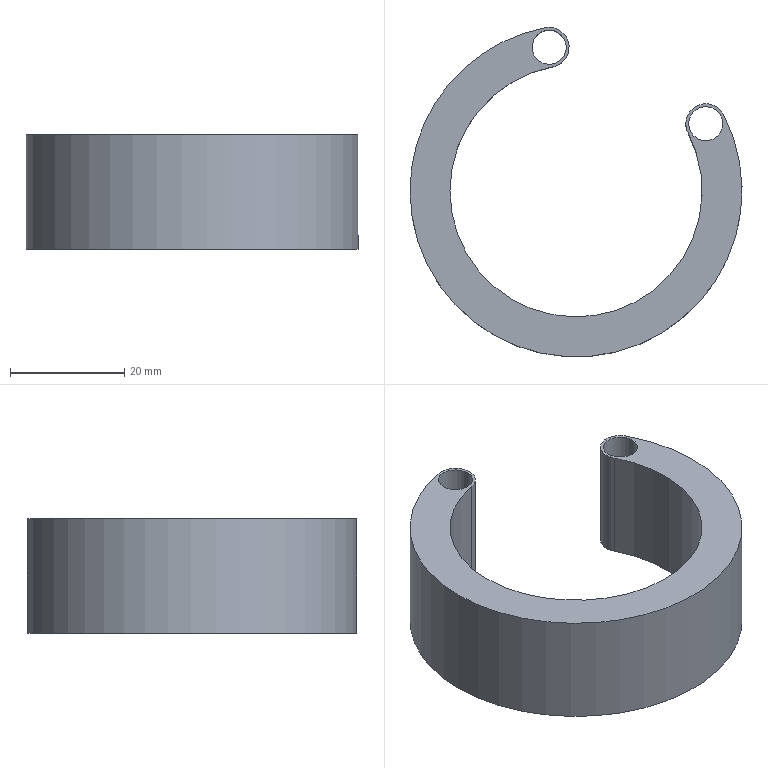Part | Creo | 1 solid | 10 faces | box 58.2 x 57.763 x 20 mm | volume 17574 mm3 | cylinder 8 | plane 2 | commonest cylinder face diameters 6 x4 7 x2 44.2 x1 58.2 x1
STEP:
#1=CARTESIAN_POINT('',(0.,0.,0.));
#2=DIRECTION('',(0.,0.,1.));
#3=DIRECTION('',(1.,0.,0.));
#4=AXIS2_PLACEMENT_3D('',#1,#2,#3);
#5=CARTESIAN_POINT('',(19.633,0.1464,85.91));
#6=VERTEX_POINT('',#5);
#7=CARTESIAN_POINT('',(-22.1,-10.,85.91));
#8=VERTEX_POINT('',#7);
#9=CARTESIAN_POINT('',(0.,-10.,85.91));
#10=DIRECTION('',(0.,0.,-1.));
#11=DIRECTION('',(0.8884,0.4591,0.));
#12=AXIS2_PLACEMENT_3D('',#9,#10,#11);
#13=CIRCLE('',#12,22.1);
#14=EDGE_CURVE('',#6,#8,#13,.T.);
#15=ORIENTED_EDGE('',*,*,#14,.F.);
#16=CARTESIAN_POINT('',(19.242,1.753,85.91));
#17=VERTEX_POINT('',#16);
#18=CARTESIAN_POINT('',(22.742,1.753,85.91));
#19=DIRECTION('',(0.,0.,1.));
#20=DIRECTION('',(-1.,0.,0.));
#21=AXIS2_PLACEMENT_3D('',#18,#19,#20);
#22=CIRCLE('',#21,3.5);
#23=EDGE_CURVE('',#17,#6,#22,.T.);
#24=ORIENTED_EDGE('',*,*,#23,.F.);
#25=CARTESIAN_POINT('',(25.852,3.36,85.91));
#26=VERTEX_POINT('',#25);
#27=CARTESIAN_POINT('',(22.742,1.753,85.91));
#28=DIRECTION('',(0.,0.,1.));
#29=DIRECTION('',(0.8884,0.4591,0.));
#30=AXIS2_PLACEMENT_3D('',#27,#28,#29);
#31=CIRCLE('',#30,3.5);
#32=EDGE_CURVE('',#26,#17,#31,.T.);
#33=ORIENTED_EDGE('',*,*,#32,.F.);
#34=CARTESIAN_POINT('',(-29.1,-10.,85.91));
#35=VERTEX_POINT('',#34);
#36=CARTESIAN_POINT('',(0.,-10.,85.91));
#37=DIRECTION('',(0.,0.,1.));
#38=DIRECTION('',(-1.,0.,0.));
#39=AXIS2_PLACEMENT_3D('',#36,#37,#38);
#40=CIRCLE('',#39,29.1);
#41=EDGE_CURVE('',#35,#26,#40,.T.);
#42=ORIENTED_EDGE('',*,*,#41,.F.);
#43=CARTESIAN_POINT('',(-5.357,18.603,85.91));
#44=VERTEX_POINT('',#43);
#45=CARTESIAN_POINT('',(0.,-10.,85.91));
#46=DIRECTION('',(0.,0.,1.));
#47=DIRECTION('',(-0.1841,0.9829,0.));
#48=AXIS2_PLACEMENT_3D('',#45,#46,#47);
#49=CIRCLE('',#48,29.1);
#50=EDGE_CURVE('',#44,#35,#49,.T.);
#51=ORIENTED_EDGE('',*,*,#50,.F.);
#52=CARTESIAN_POINT('',(-4.068,11.722,85.91));
#53=VERTEX_POINT('',#52);
#54=CARTESIAN_POINT('',(-4.712,15.163,85.91));
#55=DIRECTION('',(0.,0.,1.));
#56=DIRECTION('',(0.1841,-0.9829,0.));
#57=AXIS2_PLACEMENT_3D('',#54,#55,#56);
#58=CIRCLE('',#57,3.5);
#59=EDGE_CURVE('',#53,#44,#58,.T.);
#60=ORIENTED_EDGE('',*,*,#59,.F.);
#61=CARTESIAN_POINT('',(0.,-10.,85.91));
#62=DIRECTION('',(0.,0.,-1.));
#63=DIRECTION('',(-1.,0.,0.));
#64=AXIS2_PLACEMENT_3D('',#61,#62,#63);
#65=CIRCLE('',#64,22.1);
#66=EDGE_CURVE('',#8,#53,#65,.T.);
#67=ORIENTED_EDGE('',*,*,#66,.F.);
#68=EDGE_LOOP('',(#15,#24,#33,#42,#51,#60,#67));
#69=FACE_OUTER_BOUND('',#68,.F.);
#70=CARTESIAN_POINT('',(25.742,1.753,85.91));
#71=VERTEX_POINT('',#70);
#72=CARTESIAN_POINT('',(19.742,1.753,85.91));
#73=VERTEX_POINT('',#72);
#74=CARTESIAN_POINT('',(22.742,1.753,85.91));
#75=DIRECTION('',(0.,0.,-1.));
#76=DIRECTION('',(1.,0.,0.));
#77=AXIS2_PLACEMENT_3D('',#74,#75,#76);
#78=CIRCLE('',#77,3.);
#79=EDGE_CURVE('',#71,#73,#78,.T.);
#80=ORIENTED_EDGE('',*,*,#79,.F.);
#81=CARTESIAN_POINT('',(22.742,1.753,85.91));
#82=DIRECTION('',(0.,0.,-1.));
#83=DIRECTION('',(-1.,0.,0.));
#84=AXIS2_PLACEMENT_3D('',#81,#82,#83);
#85=CIRCLE('',#84,3.);
#86=EDGE_CURVE('',#73,#71,#85,.T.);
#87=ORIENTED_EDGE('',*,*,#86,.F.);
#88=EDGE_LOOP('',(#80,#87));
#89=FACE_BOUND('',#88,.F.);
#90=CARTESIAN_POINT('',(-1.712,15.163,85.91));
#91=VERTEX_POINT('',#90);
#92=CARTESIAN_POINT('',(-7.712,15.163,85.91));
#93=VERTEX_POINT('',#92);
#94=CARTESIAN_POINT('',(-4.712,15.163,85.91));
#95=DIRECTION('',(0.,0.,-1.));
#96=DIRECTION('',(1.,0.,0.));
#97=AXIS2_PLACEMENT_3D('',#94,#95,#96);
#98=CIRCLE('',#97,3.);
#99=EDGE_CURVE('',#91,#93,#98,.T.);
#100=ORIENTED_EDGE('',*,*,#99,.F.);
#101=CARTESIAN_POINT('',(-4.712,15.163,85.91));
#102=DIRECTION('',(0.,0.,-1.));
#103=DIRECTION('',(-1.,0.,0.));
#104=AXIS2_PLACEMENT_3D('',#101,#102,#103);
#105=CIRCLE('',#104,3.);
#106=EDGE_CURVE('',#93,#91,#105,.T.);
#107=ORIENTED_EDGE('',*,*,#106,.F.);
#108=EDGE_LOOP('',(#100,#107));
#109=FACE_BOUND('',#108,.F.);
#110=CARTESIAN_POINT('',(62.144,-0.4125,85.91));
#111=DIRECTION('',(0.,0.,1.));
#112=DIRECTION('',(0.,1.,0.));
#113=AXIS2_PLACEMENT_3D('',#110,#111,#112);
#114=PLANE('',#113);
#115=ADVANCED_FACE('',(#69,#89,#109),#114,.T.);
#116=CARTESIAN_POINT('',(-7.712,15.163,65.91));
#117=VERTEX_POINT('',#116);
#118=CARTESIAN_POINT('',(-1.712,15.163,65.91));
#119=VERTEX_POINT('',#118);
#120=CARTESIAN_POINT('',(-4.712,15.163,65.91));
#121=DIRECTION('',(0.,0.,1.));
#122=DIRECTION('',(-1.,0.,0.));
#123=AXIS2_PLACEMENT_3D('',#120,#121,#122);
#124=CIRCLE('',#123,3.);
#125=EDGE_CURVE('',#117,#119,#124,.T.);
#126=ORIENTED_EDGE('',*,*,#125,.T.);
#127=CARTESIAN_POINT('',(-1.712,15.163,85.91));
#128=DIRECTION('',(0.,0.,-1.));
#129=VECTOR('',#128,20.);
#130=LINE('',#127,#129);
#131=EDGE_CURVE('',#91,#119,#130,.T.);
#132=ORIENTED_EDGE('',*,*,#131,.F.);
#133=ORIENTED_EDGE('',*,*,#99,.T.);
#134=CARTESIAN_POINT('',(-7.712,15.163,85.91));
#135=DIRECTION('',(0.,0.,-1.));
#136=VECTOR('',#135,20.);
#137=LINE('',#134,#136);
#138=EDGE_CURVE('',#93,#117,#137,.T.);
#139=ORIENTED_EDGE('',*,*,#138,.T.);
#140=EDGE_LOOP('',(#126,#132,#133,#139));
#141=FACE_OUTER_BOUND('',#140,.F.);
#142=CARTESIAN_POINT('',(-4.712,15.163,100.91));
#143=DIRECTION('',(0.,0.,-1.));
#144=DIRECTION('',(-1.,0.,0.));
#145=AXIS2_PLACEMENT_3D('',#142,#143,#144);
#146=CYLINDRICAL_SURFACE('',#145,3.);
#147=ADVANCED_FACE('',(#141),#146,.F.);
#148=CARTESIAN_POINT('',(19.633,0.1464,65.91));
#149=VERTEX_POINT('',#148);
#150=CARTESIAN_POINT('',(19.242,1.753,65.91));
#151=VERTEX_POINT('',#150);
#152=CARTESIAN_POINT('',(22.742,1.753,65.91));
#153=DIRECTION('',(0.,0.,-1.));
#154=DIRECTION('',(-0.8884,-0.4591,0.));
#155=AXIS2_PLACEMENT_3D('',#152,#153,#154);
#156=CIRCLE('',#155,3.5);
#157=EDGE_CURVE('',#149,#151,#156,.T.);
#158=ORIENTED_EDGE('',*,*,#157,.F.);
#159=CARTESIAN_POINT('',(-22.1,-10.,65.91));
#160=VERTEX_POINT('',#159);
#161=CARTESIAN_POINT('',(0.,-10.,65.91));
#162=DIRECTION('',(0.,0.,1.));
#163=DIRECTION('',(-1.,0.,0.));
#164=AXIS2_PLACEMENT_3D('',#161,#162,#163);
#165=CIRCLE('',#164,22.1);
#166=EDGE_CURVE('',#160,#149,#165,.T.);
#167=ORIENTED_EDGE('',*,*,#166,.F.);
#168=CARTESIAN_POINT('',(-4.068,11.722,65.91));
#169=VERTEX_POINT('',#168);
#170=CARTESIAN_POINT('',(0.,-10.,65.91));
#171=DIRECTION('',(0.,0.,1.));
#172=DIRECTION('',(-0.1841,0.9829,0.));
#173=AXIS2_PLACEMENT_3D('',#170,#171,#172);
#174=CIRCLE('',#173,22.1);
#175=EDGE_CURVE('',#169,#160,#174,.T.);
#176=ORIENTED_EDGE('',*,*,#175,.F.);
#177=CARTESIAN_POINT('',(-5.357,18.603,65.91));
#178=VERTEX_POINT('',#177);
#179=CARTESIAN_POINT('',(-4.712,15.163,65.91));
#180=DIRECTION('',(0.,0.,-1.));
#181=DIRECTION('',(-0.1841,0.9829,0.));
#182=AXIS2_PLACEMENT_3D('',#179,#180,#181);
#183=CIRCLE('',#182,3.5);
#184=EDGE_CURVE('',#178,#169,#183,.T.);
#185=ORIENTED_EDGE('',*,*,#184,.F.);
#186=CARTESIAN_POINT('',(-29.1,-10.,65.91));
#187=VERTEX_POINT('',#186);
#188=CARTESIAN_POINT('',(0.,-10.,65.91));
#189=DIRECTION('',(0.,0.,-1.));
#190=DIRECTION('',(-1.,0.,0.));
#191=AXIS2_PLACEMENT_3D('',#188,#189,#190);
#192=CIRCLE('',#191,29.1);
#193=EDGE_CURVE('',#187,#178,#192,.T.);
#194=ORIENTED_EDGE('',*,*,#193,.F.);
#195=CARTESIAN_POINT('',(25.852,3.36,65.91));
#196=VERTEX_POINT('',#195);
#197=CARTESIAN_POINT('',(0.,-10.,65.91));
#198=DIRECTION('',(0.,0.,-1.));
#199=DIRECTION('',(0.8884,0.4591,0.));
#200=AXIS2_PLACEMENT_3D('',#197,#198,#199);
#201=CIRCLE('',#200,29.1);
#202=EDGE_CURVE('',#196,#187,#201,.T.);
#203=ORIENTED_EDGE('',*,*,#202,.F.);
#204=CARTESIAN_POINT('',(22.742,1.753,65.91));
#205=DIRECTION('',(0.,0.,-1.));
#206=DIRECTION('',(-1.,0.,0.));
#207=AXIS2_PLACEMENT_3D('',#204,#205,#206);
#208=CIRCLE('',#207,3.5);
#209=EDGE_CURVE('',#151,#196,#208,.T.);
#210=ORIENTED_EDGE('',*,*,#209,.F.);
#211=EDGE_LOOP('',(#158,#167,#176,#185,#194,#203,#210));
#212=FACE_OUTER_BOUND('',#211,.F.);
#213=CARTESIAN_POINT('',(25.742,1.753,65.91));
#214=VERTEX_POINT('',#213);
#215=CARTESIAN_POINT('',(19.742,1.753,65.91));
#216=VERTEX_POINT('',#215);
#217=CARTESIAN_POINT('',(22.742,1.753,65.91));
#218=DIRECTION('',(0.,0.,1.));
#219=DIRECTION('',(1.,0.,0.));
#220=AXIS2_PLACEMENT_3D('',#217,#218,#219);
#221=CIRCLE('',#220,3.);
#222=EDGE_CURVE('',#214,#216,#221,.T.);
#223=ORIENTED_EDGE('',*,*,#222,.F.);
#224=CARTESIAN_POINT('',(22.742,1.753,65.91));
#225=DIRECTION('',(0.,0.,1.));
#226=DIRECTION('',(-1.,0.,0.));
#227=AXIS2_PLACEMENT_3D('',#224,#225,#226);
#228=CIRCLE('',#227,3.);
#229=EDGE_CURVE('',#216,#214,#228,.T.);
#230=ORIENTED_EDGE('',*,*,#229,.F.);
#231=EDGE_LOOP('',(#223,#230));
#232=FACE_BOUND('',#231,.F.);
#233=CARTESIAN_POINT('',(-4.712,15.163,65.91));
#234=DIRECTION('',(0.,0.,1.));
#235=DIRECTION('',(1.,0.,0.));
#236=AXIS2_PLACEMENT_3D('',#233,#234,#235);
#237=CIRCLE('',#236,3.);
#238=EDGE_CURVE('',#119,#117,#237,.T.);
#239=ORIENTED_EDGE('',*,*,#238,.F.);
#240=ORIENTED_EDGE('',*,*,#125,.F.);
#241=EDGE_LOOP('',(#239,#240));
#242=FACE_BOUND('',#241,.F.);
#243=CARTESIAN_POINT('',(0.,0.,65.91));
#244=DIRECTION('',(0.,0.,1.));
#245=DIRECTION('',(1.,0.,0.));
#246=AXIS2_PLACEMENT_3D('',#243,#244,#245);
#247=PLANE('',#246);
#248=ADVANCED_FACE('',(#212,#232,#242),#247,.F.);
#249=ORIENTED_EDGE('',*,*,#238,.T.);
#250=ORIENTED_EDGE('',*,*,#138,.F.);
#251=ORIENTED_EDGE('',*,*,#106,.T.);
#252=ORIENTED_EDGE('',*,*,#131,.T.);
#253=EDGE_LOOP('',(#249,#250,#251,#252));
#254=FACE_OUTER_BOUND('',#253,.F.);
#255=CARTESIAN_POINT('',(-4.712,15.163,100.91));
#256=DIRECTION('',(0.,0.,-1.));
#257=DIRECTION('',(-1.,0.,0.));
#258=AXIS2_PLACEMENT_3D('',#255,#256,#257);
#259=CYLINDRICAL_SURFACE('',#258,3.);
#260=ADVANCED_FACE('',(#254),#259,.F.);
#261=ORIENTED_EDGE('',*,*,#222,.T.);
#262=CARTESIAN_POINT('',(19.742,1.753,85.91));
#263=DIRECTION('',(0.,0.,-1.));
#264=VECTOR('',#263,20.);
#265=LINE('',#262,#264);
#266=EDGE_CURVE('',#73,#216,#265,.T.);
#267=ORIENTED_EDGE('',*,*,#266,.F.);
#268=ORIENTED_EDGE('',*,*,#86,.T.);
#269=CARTESIAN_POINT('',(25.742,1.753,85.91));
#270=DIRECTION('',(0.,0.,-1.));
#271=VECTOR('',#270,20.);
#272=LINE('',#269,#271);
#273=EDGE_CURVE('',#71,#214,#272,.T.);
#274=ORIENTED_EDGE('',*,*,#273,.T.);
#275=EDGE_LOOP('',(#261,#267,#268,#274));
#276=FACE_OUTER_BOUND('',#275,.F.);
#277=CARTESIAN_POINT('',(22.742,1.753,100.91));
#278=DIRECTION('',(0.,0.,-1.));
#279=DIRECTION('',(-1.,0.,0.));
#280=AXIS2_PLACEMENT_3D('',#277,#278,#279);
#281=CYLINDRICAL_SURFACE('',#280,3.);
#282=ADVANCED_FACE('',(#276),#281,.F.);
#283=ORIENTED_EDGE('',*,*,#229,.T.);
#284=ORIENTED_EDGE('',*,*,#273,.F.);
#285=ORIENTED_EDGE('',*,*,#79,.T.);
#286=ORIENTED_EDGE('',*,*,#266,.T.);
#287=EDGE_LOOP('',(#283,#284,#285,#286));
#288=FACE_OUTER_BOUND('',#287,.F.);
#289=CARTESIAN_POINT('',(22.742,1.753,100.91));
#290=DIRECTION('',(0.,0.,-1.));
#291=DIRECTION('',(-1.,0.,0.));
#292=AXIS2_PLACEMENT_3D('',#289,#290,#291);
#293=CYLINDRICAL_SURFACE('',#292,3.);
#294=ADVANCED_FACE('',(#288),#293,.F.);
#295=CARTESIAN_POINT('',(25.852,3.36,65.91));
#296=DIRECTION('',(0.,0.,1.));
#297=VECTOR('',#296,20.);
#298=LINE('',#295,#297);
#299=EDGE_CURVE('',#196,#26,#298,.T.);
#300=ORIENTED_EDGE('',*,*,#299,.T.);
#301=ORIENTED_EDGE('',*,*,#32,.T.);
#302=ORIENTED_EDGE('',*,*,#23,.T.);
#303=CARTESIAN_POINT('',(19.633,0.1464,65.91));
#304=DIRECTION('',(0.,0.,1.));
#305=VECTOR('',#304,20.);
#306=LINE('',#303,#305);
#307=EDGE_CURVE('',#149,#6,#306,.T.);
#308=ORIENTED_EDGE('',*,*,#307,.F.);
#309=ORIENTED_EDGE('',*,*,#157,.T.);
#310=ORIENTED_EDGE('',*,*,#209,.T.);
#311=EDGE_LOOP('',(#300,#301,#302,#308,#309,#310));
#312=FACE_OUTER_BOUND('',#311,.F.);
#313=CARTESIAN_POINT('',(22.742,1.753,141.));
#314=DIRECTION('',(0.,0.,-1.));
#315=DIRECTION('',(-1.,0.,0.));
#316=AXIS2_PLACEMENT_3D('',#313,#314,#315);
#317=CYLINDRICAL_SURFACE('',#316,3.5);
#318=ADVANCED_FACE('',(#312),#317,.T.);
#319=CARTESIAN_POINT('',(-5.357,18.603,65.91));
#320=DIRECTION('',(0.,0.,1.));
#321=VECTOR('',#320,20.);
#322=LINE('',#319,#321);
#323=EDGE_CURVE('',#178,#44,#322,.T.);
#324=ORIENTED_EDGE('',*,*,#323,.T.);
#325=ORIENTED_EDGE('',*,*,#50,.T.);
#326=ORIENTED_EDGE('',*,*,#41,.T.);
#327=ORIENTED_EDGE('',*,*,#299,.F.);
#328=ORIENTED_EDGE('',*,*,#202,.T.);
#329=ORIENTED_EDGE('',*,*,#193,.T.);
#330=EDGE_LOOP('',(#324,#325,#326,#327,#328,#329));
#331=FACE_OUTER_BOUND('',#330,.F.);
#332=CARTESIAN_POINT('',(0.,-10.,141.));
#333=DIRECTION('',(0.,0.,-1.));
#334=DIRECTION('',(-1.,0.,0.));
#335=AXIS2_PLACEMENT_3D('',#332,#333,#334);
#336=CYLINDRICAL_SURFACE('',#335,29.1);
#337=ADVANCED_FACE('',(#331),#336,.T.);
#338=CARTESIAN_POINT('',(-4.068,11.722,65.91));
#339=DIRECTION('',(0.,0.,1.));
#340=VECTOR('',#339,20.);
#341=LINE('',#338,#340);
#342=EDGE_CURVE('',#169,#53,#341,.T.);
#343=ORIENTED_EDGE('',*,*,#342,.T.);
#344=ORIENTED_EDGE('',*,*,#59,.T.);
#345=ORIENTED_EDGE('',*,*,#323,.F.);
#346=ORIENTED_EDGE('',*,*,#184,.T.);
#347=EDGE_LOOP('',(#343,#344,#345,#346));
#348=FACE_OUTER_BOUND('',#347,.F.);
#349=CARTESIAN_POINT('',(-4.712,15.163,141.));
#350=DIRECTION('',(0.,0.,-1.));
#351=DIRECTION('',(-1.,0.,0.));
#352=AXIS2_PLACEMENT_3D('',#349,#350,#351);
#353=CYLINDRICAL_SURFACE('',#352,3.5);
#354=ADVANCED_FACE('',(#348),#353,.T.);
#355=ORIENTED_EDGE('',*,*,#307,.T.);
#356=ORIENTED_EDGE('',*,*,#14,.T.);
#357=ORIENTED_EDGE('',*,*,#66,.T.);
#358=ORIENTED_EDGE('',*,*,#342,.F.);
#359=ORIENTED_EDGE('',*,*,#175,.T.);
#360=ORIENTED_EDGE('',*,*,#166,.T.);
#361=EDGE_LOOP('',(#355,#356,#357,#358,#359,#360));
#362=FACE_OUTER_BOUND('',#361,.F.);
#363=CARTESIAN_POINT('',(0.,-10.,141.));
#364=DIRECTION('',(0.,0.,-1.));
#365=DIRECTION('',(-1.,0.,0.));
#366=AXIS2_PLACEMENT_3D('',#363,#364,#365);
#367=CYLINDRICAL_SURFACE('',#366,22.1);
#368=ADVANCED_FACE('',(#362),#367,.F.);
#369=CLOSED_SHELL('',(#115,#147,#248,#260,#282,#294,#318,#337,#354,#368));
#370=MANIFOLD_SOLID_BREP('',#369);
#371=(LENGTH_UNIT()NAMED_UNIT(*)SI_UNIT(.MILLI.,.METRE.));
#372=UNCERTAINTY_MEASURE_WITH_UNIT(LENGTH_MEASURE(0.008441),#371,'','');
#373=(NAMED_UNIT(*)PLANE_ANGLE_UNIT()SI_UNIT($,.RADIAN.));
#374=PLANE_ANGLE_MEASURE_WITH_UNIT(PLANE_ANGLE_MEASURE(0.01745),#373);
#375=(CONVERSION_BASED_UNIT('DEGREE',#374)NAMED_UNIT(*)PLANE_ANGLE_UNIT());
#376=(NAMED_UNIT(*)SI_UNIT($,.STERADIAN.)SOLID_ANGLE_UNIT());
#377=(GEOMETRIC_REPRESENTATION_CONTEXT(3)GLOBAL_UNCERTAINTY_ASSIGNED_CONTEXT((#372))GLOBAL_UNIT_ASSIGNED_CONTEXT((#371,#375,#376))REPRESENTATION_CONTEXT('',''));
#378=ADVANCED_BREP_SHAPE_REPRESENTATION('',(#4,#370),#377);